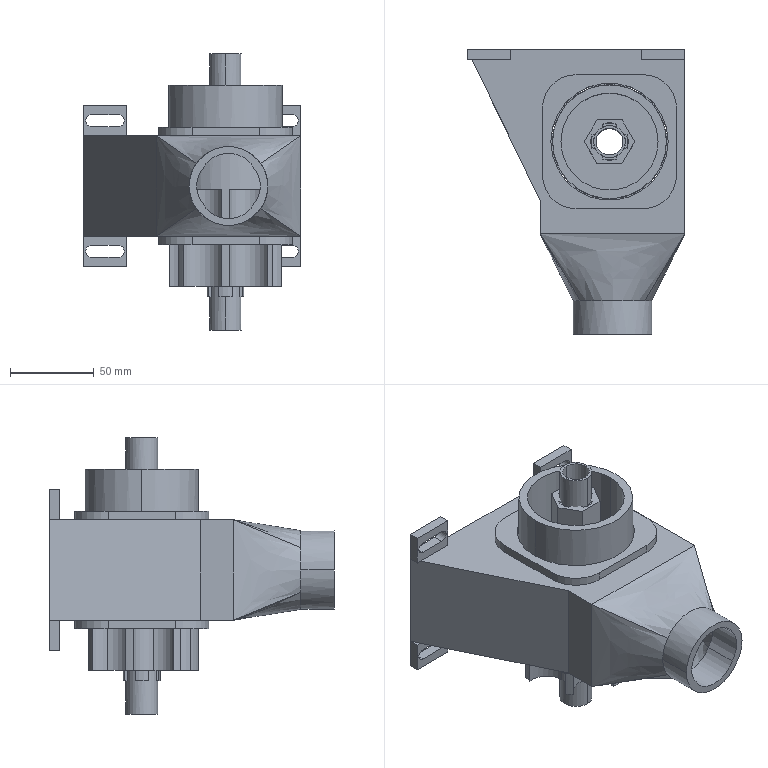Part | SolidWorks | 6 solids | 189 faces | box 130 x 170 x 165 mm | volume 426747 mm3 | plane 99 | cylinder 78 | spline 12 | commonest cylinder face diameters 70 x13 25.003 x12 25.067 x10 7 x8 40 x8 22 x5